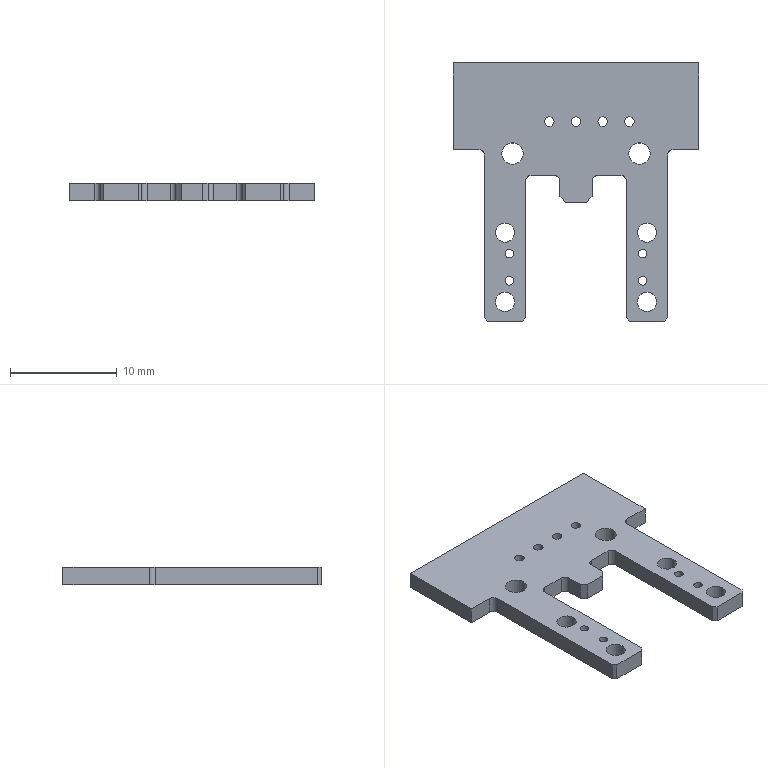Part | STEP file | 1 solid | 58 faces | box 23 x 24.2 x 1.6 mm | volume 514.519 mm3 | cylinder 34 | plane 24 | commonest cylinder face diameters 0.8 x8 0.9 x8 1.8 x8 1 x6 2 x4